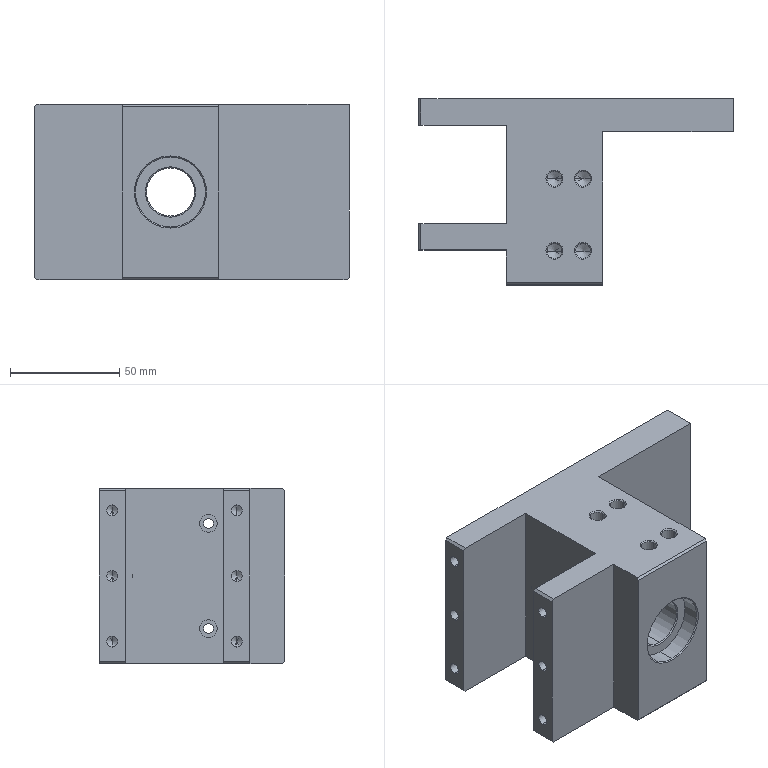Part | STEP file | longitudinal seal bearing seat_SUS304 | 1 solid | 133 faces | box 143.7 x 85 x 80 mm | volume 392938 mm3 | cone 56 | cylinder 50 | plane 27 | commonest cylinder face diameters 5 x12 6.8 x12 3.3 x8 4.5 x4 8 x4 12 x4